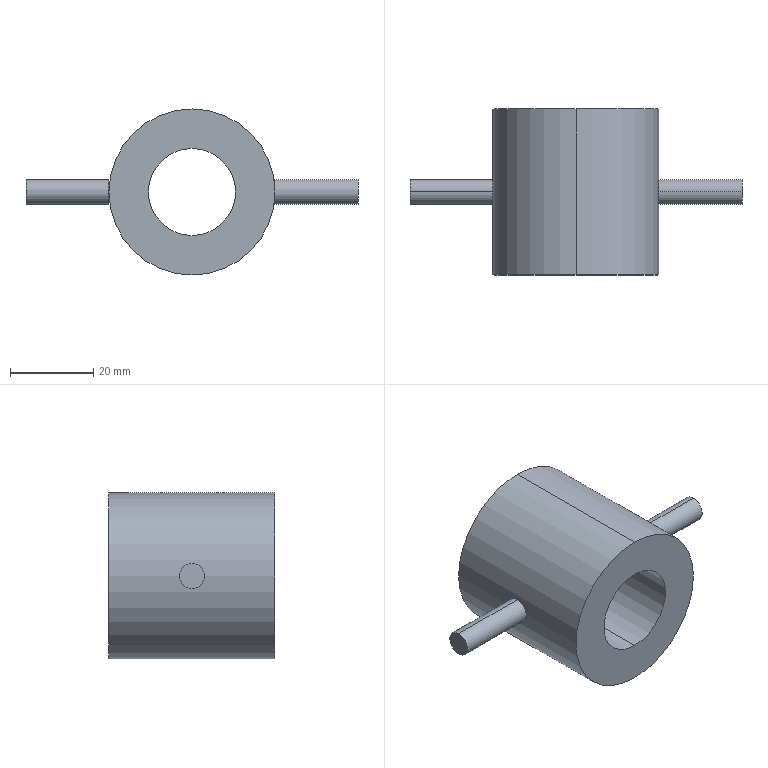Part | SolidWorks | features Extrusion 1, ICE 1, MirrorSolid 1 | 3 solids | 14 faces | box 80 x 40 x 40 mm | volume 37542 mm3 | cylinder 8 | plane 6 | commonest cylinder face diameters 6 x4 21 x2 40 x2
STEP:
#1=CARTESIAN_POINT('',(0.,40.,-10.5));
#2=VERTEX_POINT('',#1);
#3=CARTESIAN_POINT('',(0.,40.,10.5));
#4=VERTEX_POINT('',#3);
#5=CARTESIAN_POINT('',(0.,40.,0.));
#6=DIRECTION('',(0.,1.,0.));
#7=DIRECTION('',(0.,0.,1.));
#8=AXIS2_PLACEMENT_3D('',#5,#6,#7);
#9=CIRCLE('',#8,10.5);
#10=EDGE_CURVE('',#2,#4,#9,.T.);
#11=ORIENTED_EDGE('',*,*,#10,.T.);
#12=CARTESIAN_POINT('',(0.,0.,10.5));
#13=VERTEX_POINT('',#12);
#14=CARTESIAN_POINT('',(0.,40.,10.5));
#15=DIRECTION('',(0.,-1.,0.));
#16=VECTOR('',#15,1000.);
#17=LINE('',#14,#16);
#18=EDGE_CURVE('',#4,#13,#17,.T.);
#19=ORIENTED_EDGE('',*,*,#18,.T.);
#20=CARTESIAN_POINT('',(0.,0.,-10.5));
#21=VERTEX_POINT('',#20);
#22=CARTESIAN_POINT('',(0.,0.,0.));
#23=DIRECTION('',(0.,1.,0.));
#24=DIRECTION('',(0.,0.,1.));
#25=AXIS2_PLACEMENT_3D('',#22,#23,#24);
#26=CIRCLE('',#25,10.5);
#27=EDGE_CURVE('',#21,#13,#26,.T.);
#28=ORIENTED_EDGE('',*,*,#27,.F.);
#29=CARTESIAN_POINT('',(0.,40.,-10.5));
#30=DIRECTION('',(0.,-1.,0.));
#31=VECTOR('',#30,1000.);
#32=LINE('',#29,#31);
#33=EDGE_CURVE('',#2,#21,#32,.T.);
#34=ORIENTED_EDGE('',*,*,#33,.F.);
#35=EDGE_LOOP('',(#11,#19,#28,#34));
#36=FACE_OUTER_BOUND('',#35,.T.);
#37=CARTESIAN_POINT('',(0.,40.,0.));
#38=DIRECTION('',(0.,-1.,0.));
#39=DIRECTION('',(0.,0.,-1.));
#40=AXIS2_PLACEMENT_3D('',#37,#38,#39);
#41=CYLINDRICAL_SURFACE('',#40,10.5);
#42=ADVANCED_FACE('',(#36),#41,.F.);
#43=CARTESIAN_POINT('',(0.,40.,20.));
#44=VERTEX_POINT('',#43);
#45=CARTESIAN_POINT('',(0.,40.,-20.));
#46=VERTEX_POINT('',#45);
#47=CARTESIAN_POINT('',(0.,40.,0.));
#48=DIRECTION('',(0.,1.,0.));
#49=DIRECTION('',(0.,0.,1.));
#50=AXIS2_PLACEMENT_3D('',#47,#48,#49);
#51=CIRCLE('',#50,20.);
#52=EDGE_CURVE('',#44,#46,#51,.T.);
#53=ORIENTED_EDGE('',*,*,#52,.F.);
#54=CARTESIAN_POINT('',(0.,0.,20.));
#55=VERTEX_POINT('',#54);
#56=CARTESIAN_POINT('',(0.,40.,20.));
#57=DIRECTION('',(0.,-1.,0.));
#58=VECTOR('',#57,1000.);
#59=LINE('',#56,#58);
#60=EDGE_CURVE('',#44,#55,#59,.T.);
#61=ORIENTED_EDGE('',*,*,#60,.T.);
#62=CARTESIAN_POINT('',(0.,0.,-20.));
#63=VERTEX_POINT('',#62);
#64=CARTESIAN_POINT('',(0.,0.,0.));
#65=DIRECTION('',(0.,1.,0.));
#66=DIRECTION('',(0.,0.,1.));
#67=AXIS2_PLACEMENT_3D('',#64,#65,#66);
#68=CIRCLE('',#67,20.);
#69=EDGE_CURVE('',#55,#63,#68,.T.);
#70=ORIENTED_EDGE('',*,*,#69,.T.);
#71=CARTESIAN_POINT('',(0.,40.,-20.));
#72=DIRECTION('',(0.,-1.,0.));
#73=VECTOR('',#72,1000.);
#74=LINE('',#71,#73);
#75=EDGE_CURVE('',#46,#63,#74,.T.);
#76=ORIENTED_EDGE('',*,*,#75,.F.);
#77=EDGE_LOOP('',(#53,#61,#70,#76));
#78=FACE_OUTER_BOUND('',#77,.T.);
#79=CARTESIAN_POINT('',(0.,40.,0.));
#80=DIRECTION('',(0.,-1.,0.));
#81=DIRECTION('',(0.,0.,-1.));
#82=AXIS2_PLACEMENT_3D('',#79,#80,#81);
#83=CYLINDRICAL_SURFACE('',#82,20.);
#84=ADVANCED_FACE('',(#78),#83,.T.);
#85=CARTESIAN_POINT('',(0.,40.,0.));
#86=DIRECTION('',(0.,1.,0.));
#87=DIRECTION('',(0.,0.,1.));
#88=AXIS2_PLACEMENT_3D('',#85,#86,#87);
#89=CIRCLE('',#88,20.);
#90=EDGE_CURVE('',#46,#44,#89,.T.);
#91=ORIENTED_EDGE('',*,*,#90,.T.);
#92=ORIENTED_EDGE('',*,*,#52,.T.);
#93=EDGE_LOOP('',(#91,#92));
#94=FACE_OUTER_BOUND('',#93,.T.);
#95=ORIENTED_EDGE('',*,*,#10,.F.);
#96=CARTESIAN_POINT('',(0.,40.,0.));
#97=DIRECTION('',(0.,1.,0.));
#98=DIRECTION('',(0.,0.,1.));
#99=AXIS2_PLACEMENT_3D('',#96,#97,#98);
#100=CIRCLE('',#99,10.5);
#101=EDGE_CURVE('',#4,#2,#100,.T.);
#102=ORIENTED_EDGE('',*,*,#101,.F.);
#103=EDGE_LOOP('',(#95,#102));
#104=FACE_BOUND('',#103,.T.);
#105=CARTESIAN_POINT('',(0.,40.,0.));
#106=DIRECTION('',(0.,1.,0.));
#107=DIRECTION('',(0.,0.,1.));
#108=AXIS2_PLACEMENT_3D('',#105,#106,#107);
#109=PLANE('',#108);
#110=ADVANCED_FACE('',(#94,#104),#109,.T.);
#111=CARTESIAN_POINT('',(0.,0.,0.));
#112=DIRECTION('',(0.,1.,0.));
#113=DIRECTION('',(0.,0.,1.));
#114=AXIS2_PLACEMENT_3D('',#111,#112,#113);
#115=CIRCLE('',#114,20.);
#116=EDGE_CURVE('',#63,#55,#115,.T.);
#117=ORIENTED_EDGE('',*,*,#116,.F.);
#118=ORIENTED_EDGE('',*,*,#69,.F.);
#119=EDGE_LOOP('',(#117,#118));
#120=FACE_OUTER_BOUND('',#119,.T.);
#121=ORIENTED_EDGE('',*,*,#27,.T.);
#122=CARTESIAN_POINT('',(0.,0.,0.));
#123=DIRECTION('',(0.,1.,0.));
#124=DIRECTION('',(0.,0.,1.));
#125=AXIS2_PLACEMENT_3D('',#122,#123,#124);
#126=CIRCLE('',#125,10.5);
#127=EDGE_CURVE('',#13,#21,#126,.T.);
#128=ORIENTED_EDGE('',*,*,#127,.T.);
#129=EDGE_LOOP('',(#121,#128));
#130=FACE_BOUND('',#129,.T.);
#131=CARTESIAN_POINT('',(0.,0.,0.));
#132=DIRECTION('',(0.,1.,0.));
#133=DIRECTION('',(0.,0.,1.));
#134=AXIS2_PLACEMENT_3D('',#131,#132,#133);
#135=PLANE('',#134);
#136=ADVANCED_FACE('',(#120,#130),#135,.F.);
#137=ORIENTED_EDGE('',*,*,#60,.F.);
#138=ORIENTED_EDGE('',*,*,#90,.F.);
#139=ORIENTED_EDGE('',*,*,#75,.T.);
#140=ORIENTED_EDGE('',*,*,#116,.T.);
#141=EDGE_LOOP('',(#137,#138,#139,#140));
#142=FACE_OUTER_BOUND('',#141,.T.);
#143=CARTESIAN_POINT('',(0.,40.,0.));
#144=DIRECTION('',(0.,-1.,0.));
#145=DIRECTION('',(0.,0.,-1.));
#146=AXIS2_PLACEMENT_3D('',#143,#144,#145);
#147=CYLINDRICAL_SURFACE('',#146,20.);
#148=ADVANCED_FACE('',(#142),#147,.T.);
#149=ORIENTED_EDGE('',*,*,#18,.F.);
#150=ORIENTED_EDGE('',*,*,#101,.T.);
#151=ORIENTED_EDGE('',*,*,#33,.T.);
#152=ORIENTED_EDGE('',*,*,#127,.F.);
#153=EDGE_LOOP('',(#149,#150,#151,#152));
#154=FACE_OUTER_BOUND('',#153,.T.);
#155=CARTESIAN_POINT('',(0.,40.,0.));
#156=DIRECTION('',(0.,-1.,0.));
#157=DIRECTION('',(0.,0.,-1.));
#158=AXIS2_PLACEMENT_3D('',#155,#156,#157);
#159=CYLINDRICAL_SURFACE('',#158,10.5);
#160=ADVANCED_FACE('',(#154),#159,.F.);
#161=CLOSED_SHELL('',(#42,#84,#110,#136,#148,#160));
#162=MANIFOLD_SOLID_BREP('',#161);
#163=CARTESIAN_POINT('',(-40.,20.,3.));
#164=VERTEX_POINT('',#163);
#165=CARTESIAN_POINT('',(-40.,20.,-3.));
#166=VERTEX_POINT('',#165);
#167=CARTESIAN_POINT('',(-40.,20.,0.));
#168=DIRECTION('',(-1.,0.,0.));
#169=DIRECTION('',(0.,0.,1.));
#170=AXIS2_PLACEMENT_3D('',#167,#168,#169);
#171=CIRCLE('',#170,3.);
#172=EDGE_CURVE('',#164,#166,#171,.T.);
#173=ORIENTED_EDGE('',*,*,#172,.F.);
#174=CARTESIAN_POINT('',(-20.,20.,3.));
#175=VERTEX_POINT('',#174);
#176=CARTESIAN_POINT('',(-40.,20.,3.));
#177=DIRECTION('',(1.,0.,0.));
#178=VECTOR('',#177,1000.);
#179=LINE('',#176,#178);
#180=EDGE_CURVE('',#164,#175,#179,.T.);
#181=ORIENTED_EDGE('',*,*,#180,.T.);
#182=CARTESIAN_POINT('',(-20.,20.,-3.));
#183=VERTEX_POINT('',#182);
#184=CARTESIAN_POINT('',(-20.,20.,0.));
#185=DIRECTION('',(-1.,0.,0.));
#186=DIRECTION('',(0.,0.,1.));
#187=AXIS2_PLACEMENT_3D('',#184,#185,#186);
#188=CIRCLE('',#187,3.);
#189=EDGE_CURVE('',#175,#183,#188,.T.);
#190=ORIENTED_EDGE('',*,*,#189,.T.);
#191=CARTESIAN_POINT('',(-40.,20.,-3.));
#192=DIRECTION('',(1.,0.,0.));
#193=VECTOR('',#192,1000.);
#194=LINE('',#191,#193);
#195=EDGE_CURVE('',#166,#183,#194,.T.);
#196=ORIENTED_EDGE('',*,*,#195,.F.);
#197=EDGE_LOOP('',(#173,#181,#190,#196));
#198=FACE_OUTER_BOUND('',#197,.T.);
#199=CARTESIAN_POINT('',(-40.,20.,0.));
#200=DIRECTION('',(1.,0.,0.));
#201=DIRECTION('',(0.,0.,-1.));
#202=AXIS2_PLACEMENT_3D('',#199,#200,#201);
#203=CYLINDRICAL_SURFACE('',#202,3.);
#204=ADVANCED_FACE('',(#198),#203,.T.);
#205=ORIENTED_EDGE('',*,*,#180,.F.);
#206=CARTESIAN_POINT('',(-40.,20.,0.));
#207=DIRECTION('',(-1.,0.,0.));
#208=DIRECTION('',(0.,0.,1.));
#209=AXIS2_PLACEMENT_3D('',#206,#207,#208);
#210=CIRCLE('',#209,3.);
#211=EDGE_CURVE('',#166,#164,#210,.T.);
#212=ORIENTED_EDGE('',*,*,#211,.F.);
#213=ORIENTED_EDGE('',*,*,#195,.T.);
#214=CARTESIAN_POINT('',(-20.,20.,0.));
#215=DIRECTION('',(-1.,0.,0.));
#216=DIRECTION('',(0.,0.,1.));
#217=AXIS2_PLACEMENT_3D('',#214,#215,#216);
#218=CIRCLE('',#217,3.);
#219=EDGE_CURVE('',#183,#175,#218,.T.);
#220=ORIENTED_EDGE('',*,*,#219,.T.);
#221=EDGE_LOOP('',(#205,#212,#213,#220));
#222=FACE_OUTER_BOUND('',#221,.T.);
#223=CARTESIAN_POINT('',(-40.,20.,0.));
#224=DIRECTION('',(1.,0.,0.));
#225=DIRECTION('',(0.,0.,-1.));
#226=AXIS2_PLACEMENT_3D('',#223,#224,#225);
#227=CYLINDRICAL_SURFACE('',#226,3.);
#228=ADVANCED_FACE('',(#222),#227,.T.);
#229=ORIENTED_EDGE('',*,*,#211,.T.);
#230=ORIENTED_EDGE('',*,*,#172,.T.);
#231=EDGE_LOOP('',(#229,#230));
#232=FACE_OUTER_BOUND('',#231,.T.);
#233=CARTESIAN_POINT('',(-40.,20.,0.));
#234=DIRECTION('',(-1.,0.,0.));
#235=DIRECTION('',(0.,0.,1.));
#236=AXIS2_PLACEMENT_3D('',#233,#234,#235);
#237=PLANE('',#236);
#238=ADVANCED_FACE('',(#232),#237,.T.);
#239=ORIENTED_EDGE('',*,*,#219,.F.);
#240=ORIENTED_EDGE('',*,*,#189,.F.);
#241=EDGE_LOOP('',(#239,#240));
#242=FACE_OUTER_BOUND('',#241,.T.);
#243=CARTESIAN_POINT('',(-20.,20.,0.));
#244=DIRECTION('',(-1.,0.,0.));
#245=DIRECTION('',(0.,0.,1.));
#246=AXIS2_PLACEMENT_3D('',#243,#244,#245);
#247=PLANE('',#246);
#248=ADVANCED_FACE('',(#242),#247,.F.);
#249=CLOSED_SHELL('',(#204,#228,#238,#248));
#250=MANIFOLD_SOLID_BREP('',#249);
#251=CARTESIAN_POINT('',(40.,20.,-3.));
#252=VERTEX_POINT('',#251);
#253=CARTESIAN_POINT('',(40.,20.,3.));
#254=VERTEX_POINT('',#253);
#255=CARTESIAN_POINT('',(40.,20.,0.));
#256=DIRECTION('',(-1.,0.,0.));
#257=DIRECTION('',(0.,0.,1.));
#258=AXIS2_PLACEMENT_3D('',#255,#256,#257);
#259=CIRCLE('',#258,3.);
#260=EDGE_CURVE('',#252,#254,#259,.T.);
#261=ORIENTED_EDGE('',*,*,#260,.T.);
#262=CARTESIAN_POINT('',(20.,20.,3.));
#263=VERTEX_POINT('',#262);
#264=CARTESIAN_POINT('',(40.,20.,3.));
#265=DIRECTION('',(-1.,0.,0.));
#266=VECTOR('',#265,1000.);
#267=LINE('',#264,#266);
#268=EDGE_CURVE('',#254,#263,#267,.T.);
#269=ORIENTED_EDGE('',*,*,#268,.T.);
#270=CARTESIAN_POINT('',(20.,20.,-3.));
#271=VERTEX_POINT('',#270);
#272=CARTESIAN_POINT('',(20.,20.,0.));
#273=DIRECTION('',(-1.,0.,0.));
#274=DIRECTION('',(0.,0.,1.));
#275=AXIS2_PLACEMENT_3D('',#272,#273,#274);
#276=CIRCLE('',#275,3.);
#277=EDGE_CURVE('',#271,#263,#276,.T.);
#278=ORIENTED_EDGE('',*,*,#277,.F.);
#279=CARTESIAN_POINT('',(40.,20.,-3.));
#280=DIRECTION('',(-1.,0.,0.));
#281=VECTOR('',#280,1000.);
#282=LINE('',#279,#281);
#283=EDGE_CURVE('',#252,#271,#282,.T.);
#284=ORIENTED_EDGE('',*,*,#283,.F.);
#285=EDGE_LOOP('',(#261,#269,#278,#284));
#286=FACE_OUTER_BOUND('',#285,.T.);
#287=CARTESIAN_POINT('',(40.,20.,0.));
#288=DIRECTION('',(-1.,0.,0.));
#289=DIRECTION('',(0.,0.,-1.));
#290=AXIS2_PLACEMENT_3D('',#287,#288,#289);
#291=CYLINDRICAL_SURFACE('',#290,3.);
#292=ADVANCED_FACE('',(#286),#291,.T.);
#293=ORIENTED_EDGE('',*,*,#268,.F.);
#294=CARTESIAN_POINT('',(40.,20.,0.));
#295=DIRECTION('',(-1.,0.,0.));
#296=DIRECTION('',(0.,0.,1.));
#297=AXIS2_PLACEMENT_3D('',#294,#295,#296);
#298=CIRCLE('',#297,3.);
#299=EDGE_CURVE('',#254,#252,#298,.T.);
#300=ORIENTED_EDGE('',*,*,#299,.T.);
#301=ORIENTED_EDGE('',*,*,#283,.T.);
#302=CARTESIAN_POINT('',(20.,20.,0.));
#303=DIRECTION('',(-1.,0.,0.));
#304=DIRECTION('',(0.,0.,1.));
#305=AXIS2_PLACEMENT_3D('',#302,#303,#304);
#306=CIRCLE('',#305,3.);
#307=EDGE_CURVE('',#263,#271,#306,.T.);
#308=ORIENTED_EDGE('',*,*,#307,.F.);
#309=EDGE_LOOP('',(#293,#300,#301,#308));
#310=FACE_OUTER_BOUND('',#309,.T.);
#311=CARTESIAN_POINT('',(40.,20.,0.));
#312=DIRECTION('',(-1.,0.,0.));
#313=DIRECTION('',(0.,0.,-1.));
#314=AXIS2_PLACEMENT_3D('',#311,#312,#313);
#315=CYLINDRICAL_SURFACE('',#314,3.);
#316=ADVANCED_FACE('',(#310),#315,.T.);
#317=ORIENTED_EDGE('',*,*,#260,.F.);
#318=ORIENTED_EDGE('',*,*,#299,.F.);
#319=EDGE_LOOP('',(#317,#318));
#320=FACE_OUTER_BOUND('',#319,.T.);
#321=CARTESIAN_POINT('',(40.,20.,0.));
#322=DIRECTION('',(1.,0.,0.));
#323=DIRECTION('',(0.,0.,1.));
#324=AXIS2_PLACEMENT_3D('',#321,#322,#323);
#325=PLANE('',#324);
#326=ADVANCED_FACE('',(#320),#325,.T.);
#327=ORIENTED_EDGE('',*,*,#277,.T.);
#328=ORIENTED_EDGE('',*,*,#307,.T.);
#329=EDGE_LOOP('',(#327,#328));
#330=FACE_OUTER_BOUND('',#329,.T.);
#331=CARTESIAN_POINT('',(20.,20.,0.));
#332=DIRECTION('',(1.,0.,0.));
#333=DIRECTION('',(0.,0.,1.));
#334=AXIS2_PLACEMENT_3D('',#331,#332,#333);
#335=PLANE('',#334);
#336=ADVANCED_FACE('',(#330),#335,.F.);
#337=CLOSED_SHELL('',(#292,#316,#326,#336));
#338=MANIFOLD_SOLID_BREP('',#337);
#339=CARTESIAN_POINT('',(0.,0.,0.));
#340=DIRECTION('',(0.,0.,1.));
#341=DIRECTION('',(1.,0.,0.));
#342=AXIS2_PLACEMENT_3D('',#339,#340,#341);
#343=(LENGTH_UNIT()NAMED_UNIT(*)SI_UNIT(.MILLI.,.METRE.));
#344=UNCERTAINTY_MEASURE_WITH_UNIT(LENGTH_MEASURE(0.00001),#343,'','');
#345=(NAMED_UNIT(*)PLANE_ANGLE_UNIT()SI_UNIT($,.RADIAN.));
#346=(NAMED_UNIT(*)SI_UNIT($,.STERADIAN.)SOLID_ANGLE_UNIT());
#347=(GEOMETRIC_REPRESENTATION_CONTEXT(3)GLOBAL_UNCERTAINTY_ASSIGNED_CONTEXT((#344))GLOBAL_UNIT_ASSIGNED_CONTEXT((#343,#345,#346))REPRESENTATION_CONTEXT('',''));
#348=ADVANCED_BREP_SHAPE_REPRESENTATION('',(#162,#250,#338,#342),#347);